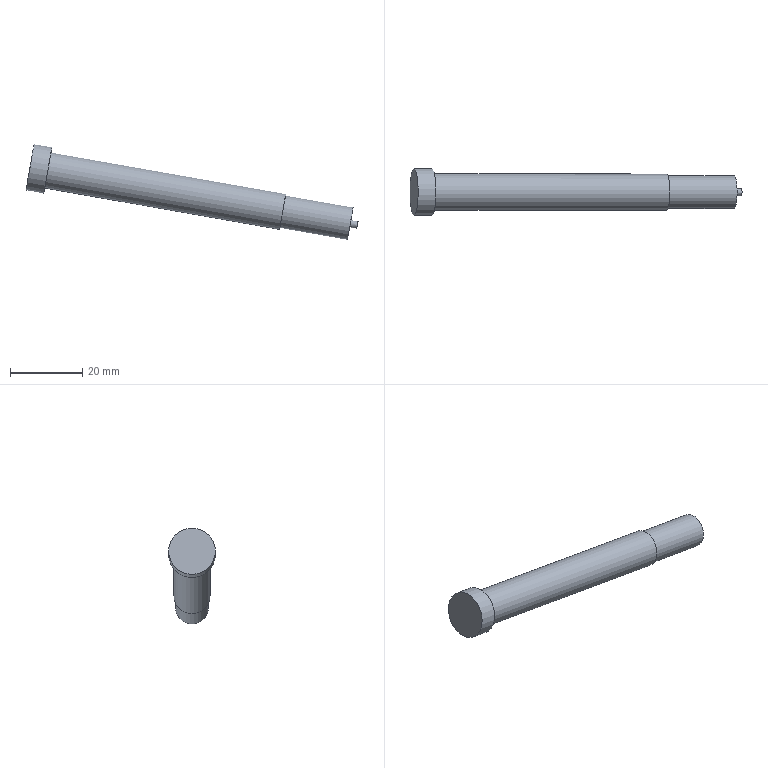Part | NX | features solid 2 | 1 solid | 9 faces | box 91.905 x 13 x 26.51 mm | volume 7089 mm3 | plane 5 | cylinder 4 | commonest cylinder face diameters 2 x1 9.1 x1 10 x1 13 x1
STEP:
#1=CARTESIAN_POINT('',(-39.657,-392.378,-34.208));
#2=VERTEX_POINT('',#1);
#3=CARTESIAN_POINT('',(-39.657,-397.378,-34.208));
#4=DIRECTION('',(0.9848,0.,-0.1736));
#5=DIRECTION('',(0.,1.,0.));
#6=AXIS2_PLACEMENT_3D('',#3,#4,#5);
#7=CIRCLE('',#6,5.);
#8=EDGE_CURVE('',#2,#2,#7,.T.);
#9=ORIENTED_EDGE('',*,*,#8,.F.);
#10=EDGE_LOOP('',(#9));
#11=FACE_BOUND('',#10,.T.);
#12=CARTESIAN_POINT('',(-104.654,-392.378,-22.747));
#13=VERTEX_POINT('',#12);
#14=CARTESIAN_POINT('',(-104.654,-397.378,-22.747));
#15=DIRECTION('',(0.9848,0.,-0.1736));
#16=DIRECTION('',(0.,1.,0.));
#17=AXIS2_PLACEMENT_3D('',#14,#15,#16);
#18=CIRCLE('',#17,5.);
#19=EDGE_CURVE('',#13,#13,#18,.T.);
#20=ORIENTED_EDGE('',*,*,#19,.T.);
#21=EDGE_LOOP('',(#20));
#22=FACE_BOUND('',#21,.T.);
#23=CARTESIAN_POINT('',(-109.578,-397.378,-21.879));
#24=DIRECTION('',(0.9848,0.,-0.1736));
#25=DIRECTION('',(0.,-1.,0.));
#26=AXIS2_PLACEMENT_3D('',#23,#24,#25);
#27=CYLINDRICAL_SURFACE('',#26,5.);
#28=ADVANCED_FACE('',(#11,#22),#27,.T.);
#29=CARTESIAN_POINT('',(-39.657,-392.828,-34.208));
#30=VERTEX_POINT('',#29);
#31=CARTESIAN_POINT('',(-39.657,-397.378,-34.208));
#32=DIRECTION('',(0.9848,0.,-0.1736));
#33=DIRECTION('',(0.,1.,0.));
#34=AXIS2_PLACEMENT_3D('',#31,#32,#33);
#35=CIRCLE('',#34,4.55);
#36=EDGE_CURVE('',#30,#30,#35,.T.);
#37=ORIENTED_EDGE('',*,*,#36,.F.);
#38=EDGE_LOOP('',(#37));
#39=FACE_BOUND('',#38,.T.);
#40=ORIENTED_EDGE('',*,*,#8,.T.);
#41=EDGE_LOOP('',(#40));
#42=FACE_BOUND('',#41,.T.);
#43=CARTESIAN_POINT('',(-39.657,-397.378,-34.208));
#44=DIRECTION('',(-0.9848,0.,0.1736));
#45=DIRECTION('',(0.,1.,0.));
#46=AXIS2_PLACEMENT_3D('',#43,#44,#45);
#47=PLANE('',#46);
#48=ADVANCED_FACE('',(#39,#42),#47,.F.);
#49=CARTESIAN_POINT('',(-104.654,-390.878,-22.747));
#50=VERTEX_POINT('',#49);
#51=CARTESIAN_POINT('',(-104.654,-397.378,-22.747));
#52=DIRECTION('',(0.9848,0.,-0.1736));
#53=DIRECTION('',(0.,1.,0.));
#54=AXIS2_PLACEMENT_3D('',#51,#52,#53);
#55=CIRCLE('',#54,6.5);
#56=EDGE_CURVE('',#50,#50,#55,.T.);
#57=ORIENTED_EDGE('',*,*,#56,.T.);
#58=EDGE_LOOP('',(#57));
#59=FACE_BOUND('',#58,.T.);
#60=ORIENTED_EDGE('',*,*,#19,.F.);
#61=EDGE_LOOP('',(#60));
#62=FACE_BOUND('',#61,.T.);
#63=CARTESIAN_POINT('',(-104.654,-397.378,-22.747));
#64=DIRECTION('',(-0.9848,0.,0.1736));
#65=DIRECTION('',(0.,1.,0.));
#66=AXIS2_PLACEMENT_3D('',#63,#64,#65);
#67=PLANE('',#66);
#68=ADVANCED_FACE('',(#59,#62),#67,.F.);
#69=ORIENTED_EDGE('',*,*,#56,.F.);
#70=EDGE_LOOP('',(#69));
#71=FACE_BOUND('',#70,.T.);
#72=CARTESIAN_POINT('',(-109.578,-390.878,-21.879));
#73=VERTEX_POINT('',#72);
#74=CARTESIAN_POINT('',(-109.578,-397.378,-21.879));
#75=DIRECTION('',(0.9848,0.,-0.1736));
#76=DIRECTION('',(0.,1.,0.));
#77=AXIS2_PLACEMENT_3D('',#74,#75,#76);
#78=CIRCLE('',#77,6.5);
#79=EDGE_CURVE('',#73,#73,#78,.T.);
#80=ORIENTED_EDGE('',*,*,#79,.T.);
#81=EDGE_LOOP('',(#80));
#82=FACE_BOUND('',#81,.T.);
#83=CARTESIAN_POINT('',(-104.654,-397.378,-22.747));
#84=DIRECTION('',(-0.9848,0.,0.1736));
#85=DIRECTION('',(0.,1.,0.));
#86=AXIS2_PLACEMENT_3D('',#83,#84,#85);
#87=CYLINDRICAL_SURFACE('',#86,6.5);
#88=ADVANCED_FACE('',(#71,#82),#87,.T.);
#89=ORIENTED_EDGE('',*,*,#79,.F.);
#90=EDGE_LOOP('',(#89));
#91=FACE_BOUND('',#90,.T.);
#92=CARTESIAN_POINT('',(-109.578,-397.378,-21.879));
#93=DIRECTION('',(-0.9848,0.,0.1736));
#94=DIRECTION('',(0.,1.,0.));
#95=AXIS2_PLACEMENT_3D('',#92,#93,#94);
#96=PLANE('',#95);
#97=ADVANCED_FACE('',(#91),#96,.T.);
#98=CARTESIAN_POINT('',(-20.945,-392.828,-37.507));
#99=VERTEX_POINT('',#98);
#100=CARTESIAN_POINT('',(-20.945,-397.378,-37.507));
#101=DIRECTION('',(0.9848,0.,-0.1736));
#102=DIRECTION('',(0.,1.,0.));
#103=AXIS2_PLACEMENT_3D('',#100,#101,#102);
#104=CIRCLE('',#103,4.55);
#105=EDGE_CURVE('',#99,#99,#104,.T.);
#106=ORIENTED_EDGE('',*,*,#105,.F.);
#107=EDGE_LOOP('',(#106));
#108=FACE_BOUND('',#107,.T.);
#109=ORIENTED_EDGE('',*,*,#36,.T.);
#110=EDGE_LOOP('',(#109));
#111=FACE_BOUND('',#110,.T.);
#112=CARTESIAN_POINT('',(-20.945,-397.378,-37.507));
#113=DIRECTION('',(-0.9848,0.,0.1736));
#114=DIRECTION('',(0.,1.,0.));
#115=AXIS2_PLACEMENT_3D('',#112,#113,#114);
#116=CYLINDRICAL_SURFACE('',#115,4.55);
#117=ADVANCED_FACE('',(#108,#111),#116,.T.);
#118=CARTESIAN_POINT('',(-20.945,-396.378,-37.507));
#119=VERTEX_POINT('',#118);
#120=CARTESIAN_POINT('',(-20.945,-397.378,-37.507));
#121=DIRECTION('',(0.9848,0.,-0.1736));
#122=DIRECTION('',(0.,1.,0.));
#123=AXIS2_PLACEMENT_3D('',#120,#121,#122);
#124=CIRCLE('',#123,1.);
#125=EDGE_CURVE('',#119,#119,#124,.T.);
#126=ORIENTED_EDGE('',*,*,#125,.F.);
#127=EDGE_LOOP('',(#126));
#128=FACE_BOUND('',#127,.T.);
#129=ORIENTED_EDGE('',*,*,#105,.T.);
#130=EDGE_LOOP('',(#129));
#131=FACE_BOUND('',#130,.T.);
#132=CARTESIAN_POINT('',(-20.945,-397.378,-37.507));
#133=DIRECTION('',(-0.9848,0.,0.1736));
#134=DIRECTION('',(0.,1.,0.));
#135=AXIS2_PLACEMENT_3D('',#132,#133,#134);
#136=PLANE('',#135);
#137=ADVANCED_FACE('',(#128,#131),#136,.F.);
#138=CARTESIAN_POINT('',(-18.976,-396.378,-37.855));
#139=VERTEX_POINT('',#138);
#140=CARTESIAN_POINT('',(-18.976,-397.378,-37.855));
#141=DIRECTION('',(0.9848,0.,-0.1736));
#142=DIRECTION('',(0.,1.,0.));
#143=AXIS2_PLACEMENT_3D('',#140,#141,#142);
#144=CIRCLE('',#143,1.);
#145=EDGE_CURVE('',#139,#139,#144,.T.);
#146=ORIENTED_EDGE('',*,*,#145,.F.);
#147=EDGE_LOOP('',(#146));
#148=FACE_BOUND('',#147,.T.);
#149=ORIENTED_EDGE('',*,*,#125,.T.);
#150=EDGE_LOOP('',(#149));
#151=FACE_BOUND('',#150,.T.);
#152=CARTESIAN_POINT('',(-18.976,-397.378,-37.855));
#153=DIRECTION('',(-0.9848,0.,0.1736));
#154=DIRECTION('',(0.,1.,0.));
#155=AXIS2_PLACEMENT_3D('',#152,#153,#154);
#156=CYLINDRICAL_SURFACE('',#155,1.);
#157=ADVANCED_FACE('',(#148,#151),#156,.T.);
#158=ORIENTED_EDGE('',*,*,#145,.T.);
#159=EDGE_LOOP('',(#158));
#160=FACE_BOUND('',#159,.T.);
#161=CARTESIAN_POINT('',(-18.976,-397.378,-37.855));
#162=DIRECTION('',(-0.9848,0.,0.1736));
#163=DIRECTION('',(0.,1.,0.));
#164=AXIS2_PLACEMENT_3D('',#161,#162,#163);
#165=PLANE('',#164);
#166=ADVANCED_FACE('',(#160),#165,.F.);
#167=CLOSED_SHELL('',(#28,#48,#68,#88,#97,#117,#137,#157,#166));
#168=MANIFOLD_SOLID_BREP('',#167);
#169=(LENGTH_UNIT()NAMED_UNIT(*)SI_UNIT(.MILLI.,.METRE.));
#170=UNCERTAINTY_MEASURE_WITH_UNIT(LENGTH_MEASURE(0.00001),#169,'','');
#171=(NAMED_UNIT(*)PLANE_ANGLE_UNIT()SI_UNIT($,.RADIAN.));
#172=(NAMED_UNIT(*)SI_UNIT($,.STERADIAN.)SOLID_ANGLE_UNIT());
#173=(GEOMETRIC_REPRESENTATION_CONTEXT(3)GLOBAL_UNCERTAINTY_ASSIGNED_CONTEXT((#170))GLOBAL_UNIT_ASSIGNED_CONTEXT((#169,#171,#172))REPRESENTATION_CONTEXT('',''));
#174=ADVANCED_BREP_SHAPE_REPRESENTATION('',(#168),#173);